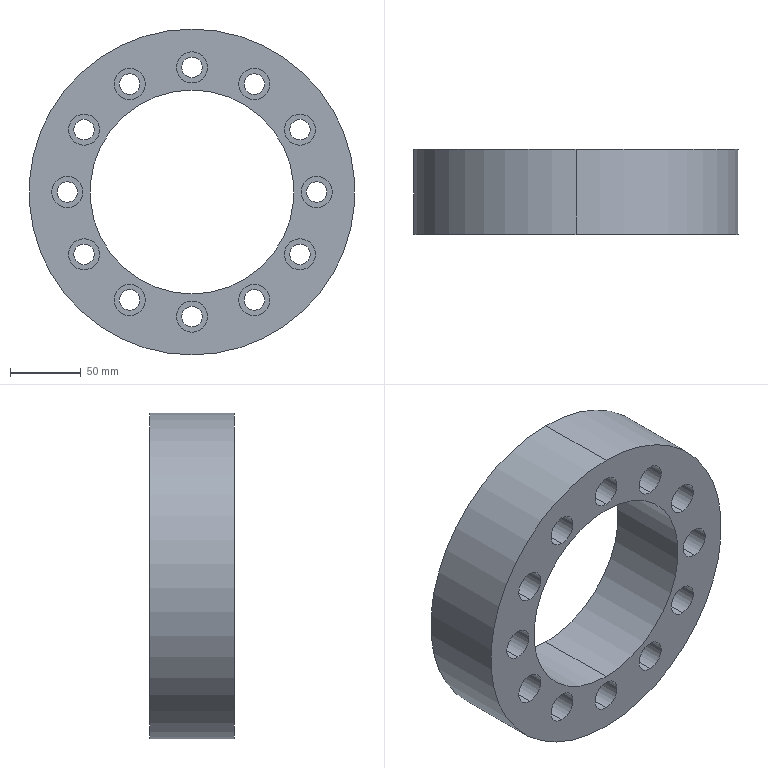Part | SolidWorks | features Extrusion 1, ICE 1 | 1 solid | 66 faces | box 230 x 60 x 230 mm | volume 1319398 mm3 | cylinder 52 | plane 14 | commonest cylinder face diameters 14.5 x24 22 x24 144 x2 230 x2